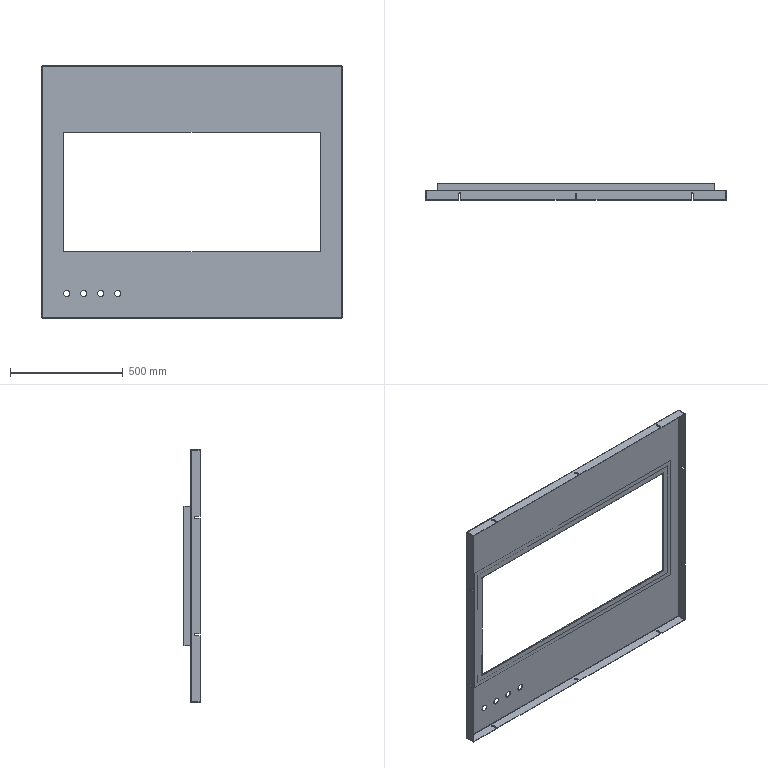Part | NX | 1 solid | 96 faces | box 1329 x 72 x 1119 mm | volume 4312851 mm3 | plane 66 | cylinder 22 | spline 8 | commonest cylinder face diameters 8.5 x10 0.4 x4 4.4 x4 27 x4